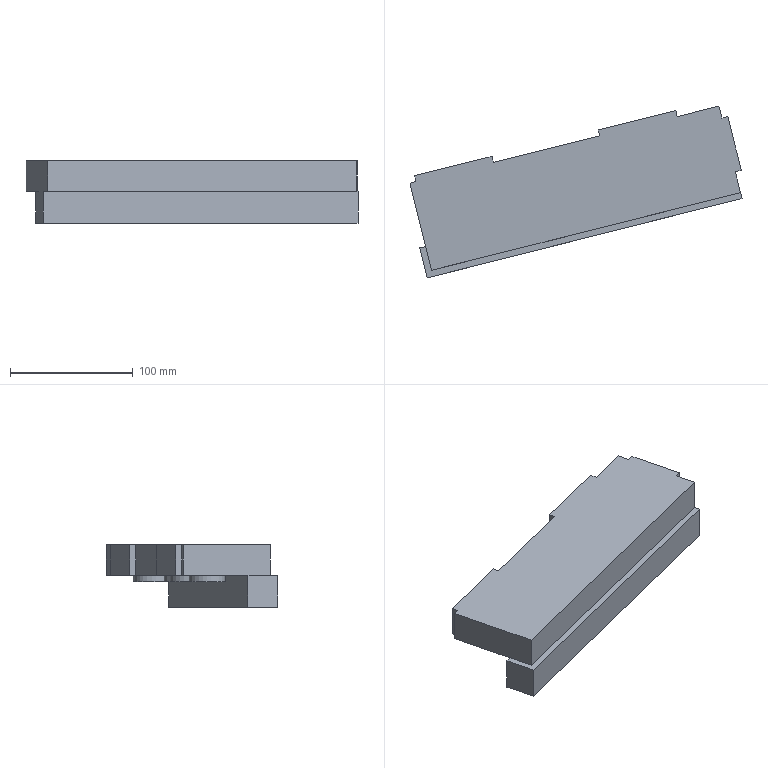Part | NX | features solid 2 | 1 solid | 33 faces | box 270.03 x 139.571 x 51 mm | volume 681907 mm3 | plane 25 | cylinder 5 | spline 3 | commonest cylinder face diameters 30 x5
STEP:
#1=CARTESIAN_POINT('',(-5.928,607.408,20.));
#2=VERTEX_POINT('',#1);
#3=CARTESIAN_POINT('',(9.072,607.408,20.));
#4=DIRECTION('',(0.,0.,-1.));
#5=DIRECTION('',(-1.,0.,0.));
#6=AXIS2_PLACEMENT_3D('',#3,#4,#5);
#7=CIRCLE('',#6,15.);
#8=EDGE_CURVE('',#2,#2,#7,.T.);
#9=ORIENTED_EDGE('',*,*,#8,.F.);
#10=EDGE_LOOP('',(#9));
#11=FACE_BOUND('',#10,.T.);
#12=CARTESIAN_POINT('',(114.072,637.408,20.));
#13=VERTEX_POINT('',#12);
#14=CARTESIAN_POINT('',(129.072,637.408,20.));
#15=DIRECTION('',(0.,0.,-1.));
#16=DIRECTION('',(-1.,0.,0.));
#17=AXIS2_PLACEMENT_3D('',#14,#15,#16);
#18=CIRCLE('',#17,15.);
#19=EDGE_CURVE('',#13,#13,#18,.T.);
#20=ORIENTED_EDGE('',*,*,#19,.F.);
#21=EDGE_LOOP('',(#20));
#22=FACE_BOUND('',#21,.T.);
#23=CARTESIAN_POINT('',(188.432,674.455,20.));
#24=VERTEX_POINT('',#23);
#25=CARTESIAN_POINT('',(154.471,665.988,20.));
#26=VERTEX_POINT('',#25);
#27=CARTESIAN_POINT('',(-67.726,610.588,20.));
#28=DIRECTION('',(0.9703,0.2419,0.));
#29=VECTOR('',#28,1000.);
#30=LINE('',#27,#29);
#31=EDGE_CURVE('',#24,#26,#30,.F.);
#32=ORIENTED_EDGE('',*,*,#31,.F.);
#33=CARTESIAN_POINT('',(190.851,664.752,20.));
#34=VERTEX_POINT('',#33);
#35=CARTESIAN_POINT('',(207.307,598.752,20.));
#36=DIRECTION('',(-0.2419,0.9703,0.));
#37=VECTOR('',#36,1000.);
#38=LINE('',#35,#37);
#39=EDGE_CURVE('',#24,#34,#38,.F.);
#40=ORIENTED_EDGE('',*,*,#39,.T.);
#41=CARTESIAN_POINT('',(195.702,665.962,20.));
#42=VERTEX_POINT('',#41);
#43=CARTESIAN_POINT('',(190.851,664.752,20.));
#44=DIRECTION('',(0.9703,0.2419,0.));
#45=VECTOR('',#44,1000.);
#46=LINE('',#43,#45);
#47=EDGE_CURVE('',#34,#42,#46,.T.);
#48=ORIENTED_EDGE('',*,*,#47,.T.);
#49=CARTESIAN_POINT('',(206.589,622.298,20.));
#50=VERTEX_POINT('',#49);
#51=CARTESIAN_POINT('',(198.122,656.259,20.));
#52=DIRECTION('',(-0.2419,0.9703,0.));
#53=VECTOR('',#52,1000.);
#54=LINE('',#51,#53);
#55=EDGE_CURVE('',#50,#42,#54,.T.);
#56=ORIENTED_EDGE('',*,*,#55,.F.);
#57=CARTESIAN_POINT('',(201.737,621.089,20.));
#58=VERTEX_POINT('',#57);
#59=CARTESIAN_POINT('',(201.737,621.089,20.));
#60=DIRECTION('',(0.9703,0.2419,0.));
#61=VECTOR('',#60,1000.);
#62=LINE('',#59,#61);
#63=EDGE_CURVE('',#58,#50,#62,.T.);
#64=ORIENTED_EDGE('',*,*,#63,.F.);
#65=CARTESIAN_POINT('',(201.108,623.615,20.));
#66=VERTEX_POINT('',#65);
#67=CARTESIAN_POINT('',(193.27,655.049,20.));
#68=DIRECTION('',(-0.2419,0.9703,0.));
#69=VECTOR('',#68,1000.);
#70=LINE('',#67,#69);
#71=EDGE_CURVE('',#58,#66,#70,.T.);
#72=ORIENTED_EDGE('',*,*,#71,.T.);
#73=CARTESIAN_POINT('',(-50.051,560.362,20.));
#74=VERTEX_POINT('',#73);
#75=CARTESIAN_POINT('',(-50.051,560.362,20.));
#76=CARTESIAN_POINT('',(33.671,581.439,20.));
#77=CARTESIAN_POINT('',(117.388,602.531,20.));
#78=CARTESIAN_POINT('',(201.108,623.615,20.));
#79=B_SPLINE_CURVE_WITH_KNOTS('',3,(#75,#76,#77,#78),.UNSPECIFIED.,.F.,.F.,(4,4),(1.461,1.72),.UNSPECIFIED.);
#80=EDGE_CURVE('',#74,#66,#79,.T.);
#81=ORIENTED_EDGE('',*,*,#80,.F.);
#82=CARTESIAN_POINT('',(-62.875,611.797,20.));
#83=VERTEX_POINT('',#82);
#84=CARTESIAN_POINT('',(-45.209,540.945,20.));
#85=DIRECTION('',(0.2419,-0.9703,0.));
#86=VECTOR('',#85,1000.);
#87=LINE('',#84,#86);
#88=EDGE_CURVE('',#74,#83,#87,.F.);
#89=ORIENTED_EDGE('',*,*,#88,.T.);
#90=CARTESIAN_POINT('',(-58.023,613.007,20.));
#91=VERTEX_POINT('',#90);
#92=CARTESIAN_POINT('',(-67.726,610.588,20.));
#93=DIRECTION('',(0.9703,0.2419,0.));
#94=VECTOR('',#93,1000.);
#95=LINE('',#92,#94);
#96=EDGE_CURVE('',#91,#83,#95,.F.);
#97=ORIENTED_EDGE('',*,*,#96,.F.);
#98=CARTESIAN_POINT('',(-59.233,617.858,20.));
#99=VERTEX_POINT('',#98);
#100=CARTESIAN_POINT('',(-58.023,613.007,20.));
#101=DIRECTION('',(-0.2419,0.9703,0.));
#102=VECTOR('',#101,1000.);
#103=LINE('',#100,#102);
#104=EDGE_CURVE('',#91,#99,#103,.T.);
#105=ORIENTED_EDGE('',*,*,#104,.T.);
#106=CARTESIAN_POINT('',(3.836,633.583,20.));
#107=VERTEX_POINT('',#106);
#108=CARTESIAN_POINT('',(-64.084,616.649,20.));
#109=DIRECTION('',(0.9703,0.2419,0.));
#110=VECTOR('',#109,1000.);
#111=LINE('',#108,#110);
#112=EDGE_CURVE('',#99,#107,#111,.T.);
#113=ORIENTED_EDGE('',*,*,#112,.T.);
#114=CARTESIAN_POINT('',(5.046,628.732,20.));
#115=VERTEX_POINT('',#114);
#116=CARTESIAN_POINT('',(5.046,628.732,20.));
#117=DIRECTION('',(-0.2419,0.9703,0.));
#118=VECTOR('',#117,1000.);
#119=LINE('',#116,#118);
#120=EDGE_CURVE('',#115,#107,#119,.T.);
#121=ORIENTED_EDGE('',*,*,#120,.F.);
#122=CARTESIAN_POINT('',(91.402,650.263,20.));
#123=VERTEX_POINT('',#122);
#124=CARTESIAN_POINT('',(-67.726,610.588,20.));
#125=DIRECTION('',(0.9703,0.2419,0.));
#126=VECTOR('',#125,1000.);
#127=LINE('',#124,#126);
#128=EDGE_CURVE('',#123,#115,#127,.F.);
#129=ORIENTED_EDGE('',*,*,#128,.F.);
#130=CARTESIAN_POINT('',(90.193,655.114,20.));
#131=VERTEX_POINT('',#130);
#132=CARTESIAN_POINT('',(91.402,650.263,20.));
#133=DIRECTION('',(-0.2419,0.9703,0.));
#134=VECTOR('',#133,1000.);
#135=LINE('',#132,#134);
#136=EDGE_CURVE('',#123,#131,#135,.T.);
#137=ORIENTED_EDGE('',*,*,#136,.T.);
#138=CARTESIAN_POINT('',(153.262,670.839,20.));
#139=VERTEX_POINT('',#138);
#140=CARTESIAN_POINT('',(129.004,664.791,20.));
#141=DIRECTION('',(0.9703,0.2419,0.));
#142=VECTOR('',#141,1000.);
#143=LINE('',#140,#142);
#144=EDGE_CURVE('',#131,#139,#143,.T.);
#145=ORIENTED_EDGE('',*,*,#144,.T.);
#146=CARTESIAN_POINT('',(154.471,665.988,20.));
#147=DIRECTION('',(-0.2419,0.9703,0.));
#148=VECTOR('',#147,1000.);
#149=LINE('',#146,#148);
#150=EDGE_CURVE('',#26,#139,#149,.T.);
#151=ORIENTED_EDGE('',*,*,#150,.F.);
#152=EDGE_LOOP('',(#32,#40,#48,#56,#64,#72,#81,#89,#97,#105,#113,#121,#129,#137,#145,#151));
#153=FACE_BOUND('',#152,.T.);
#154=CARTESIAN_POINT('',(-35.928,592.408,20.));
#155=VERTEX_POINT('',#154);
#156=CARTESIAN_POINT('',(-20.928,592.408,20.));
#157=DIRECTION('',(0.,0.,-1.));
#158=DIRECTION('',(-1.,0.,0.));
#159=AXIS2_PLACEMENT_3D('',#156,#157,#158);
#160=CIRCLE('',#159,15.);
#161=EDGE_CURVE('',#155,#155,#160,.T.);
#162=ORIENTED_EDGE('',*,*,#161,.F.);
#163=EDGE_LOOP('',(#162));
#164=FACE_BOUND('',#163,.T.);
#165=CARTESIAN_POINT('',(59.072,612.408,20.));
#166=VERTEX_POINT('',#165);
#167=CARTESIAN_POINT('',(74.072,612.408,20.));
#168=DIRECTION('',(0.,0.,-1.));
#169=DIRECTION('',(-1.,0.,0.));
#170=AXIS2_PLACEMENT_3D('',#167,#168,#169);
#171=CIRCLE('',#170,15.);
#172=EDGE_CURVE('',#166,#166,#171,.T.);
#173=ORIENTED_EDGE('',*,*,#172,.F.);
#174=EDGE_LOOP('',(#173));
#175=FACE_BOUND('',#174,.T.);
#176=CARTESIAN_POINT('',(149.072,637.408,20.));
#177=VERTEX_POINT('',#176);
#178=CARTESIAN_POINT('',(164.072,637.408,20.));
#179=DIRECTION('',(0.,0.,-1.));
#180=DIRECTION('',(-1.,0.,0.));
#181=AXIS2_PLACEMENT_3D('',#178,#179,#180);
#182=CIRCLE('',#181,15.);
#183=EDGE_CURVE('',#177,#177,#182,.T.);
#184=ORIENTED_EDGE('',*,*,#183,.F.);
#185=EDGE_LOOP('',(#184));
#186=FACE_BOUND('',#185,.T.);
#187=CARTESIAN_POINT('',(-48.851,534.884,20.));
#188=DIRECTION('',(0.,0.,-1.));
#189=DIRECTION('',(-1.,0.,0.));
#190=AXIS2_PLACEMENT_3D('',#187,#188,#189);
#191=PLANE('',#190);
#192=ADVANCED_FACE('',(#11,#22,#153,#164,#175,#186),#191,.T.);
#193=CARTESIAN_POINT('',(190.851,664.752,45.));
#194=VERTEX_POINT('',#193);
#195=CARTESIAN_POINT('',(188.432,674.455,45.));
#196=VERTEX_POINT('',#195);
#197=CARTESIAN_POINT('',(819.566,-1856.886,45.));
#198=DIRECTION('',(-0.2419,0.9703,0.));
#199=VECTOR('',#198,1000.);
#200=LINE('',#197,#199);
#201=EDGE_CURVE('',#194,#196,#200,.T.);
#202=ORIENTED_EDGE('',*,*,#201,.F.);
#203=CARTESIAN_POINT('',(190.851,664.752,20.));
#204=DIRECTION('',(0.,0.,1.));
#205=VECTOR('',#204,1000.);
#206=LINE('',#203,#205);
#207=EDGE_CURVE('',#34,#194,#206,.T.);
#208=ORIENTED_EDGE('',*,*,#207,.F.);
#209=ORIENTED_EDGE('',*,*,#39,.F.);
#210=CARTESIAN_POINT('',(188.432,674.455,70.));
#211=DIRECTION('',(0.,0.,-1.));
#212=VECTOR('',#211,1000.);
#213=LINE('',#210,#212);
#214=EDGE_CURVE('',#196,#24,#213,.T.);
#215=ORIENTED_EDGE('',*,*,#214,.F.);
#216=EDGE_LOOP('',(#202,#208,#209,#215));
#217=FACE_BOUND('',#216,.T.);
#218=CARTESIAN_POINT('',(819.566,-1856.886,70.));
#219=DIRECTION('',(-0.9703,-0.2419,0.));
#220=DIRECTION('',(0.2419,-0.9703,0.));
#221=AXIS2_PLACEMENT_3D('',#218,#219,#220);
#222=PLANE('',#221);
#223=ADVANCED_FACE('',(#217),#222,.F.);
#224=CARTESIAN_POINT('',(5.046,628.732,45.));
#225=VERTEX_POINT('',#224);
#226=CARTESIAN_POINT('',(91.402,650.263,45.));
#227=VERTEX_POINT('',#226);
#228=CARTESIAN_POINT('',(-334.558,544.059,45.));
#229=DIRECTION('',(0.9703,0.2419,0.));
#230=VECTOR('',#229,1000.);
#231=LINE('',#228,#230);
#232=EDGE_CURVE('',#225,#227,#231,.T.);
#233=ORIENTED_EDGE('',*,*,#232,.T.);
#234=CARTESIAN_POINT('',(91.402,650.263,45.));
#235=DIRECTION('',(0.,0.,1.));
#236=VECTOR('',#235,1000.);
#237=LINE('',#234,#236);
#238=EDGE_CURVE('',#227,#123,#237,.F.);
#239=ORIENTED_EDGE('',*,*,#238,.T.);
#240=ORIENTED_EDGE('',*,*,#128,.T.);
#241=CARTESIAN_POINT('',(5.046,628.732,45.));
#242=DIRECTION('',(0.,0.,-1.));
#243=VECTOR('',#242,1000.);
#244=LINE('',#241,#243);
#245=EDGE_CURVE('',#225,#115,#244,.T.);
#246=ORIENTED_EDGE('',*,*,#245,.F.);
#247=EDGE_LOOP('',(#233,#239,#240,#246));
#248=FACE_BOUND('',#247,.T.);
#249=CARTESIAN_POINT('',(-334.558,544.059,70.));
#250=DIRECTION('',(-0.2419,0.9703,0.));
#251=DIRECTION('',(-0.9703,-0.2419,0.));
#252=AXIS2_PLACEMENT_3D('',#249,#250,#251);
#253=PLANE('',#252);
#254=ADVANCED_FACE('',(#248),#253,.T.);
#255=CARTESIAN_POINT('',(-62.875,611.797,45.));
#256=VERTEX_POINT('',#255);
#257=CARTESIAN_POINT('',(-58.023,613.007,45.));
#258=VERTEX_POINT('',#257);
#259=CARTESIAN_POINT('',(-334.558,544.059,45.));
#260=DIRECTION('',(0.9703,0.2419,0.));
#261=VECTOR('',#260,1000.);
#262=LINE('',#259,#261);
#263=EDGE_CURVE('',#256,#258,#262,.T.);
#264=ORIENTED_EDGE('',*,*,#263,.T.);
#265=CARTESIAN_POINT('',(-58.023,613.007,45.));
#266=DIRECTION('',(0.,0.,1.));
#267=VECTOR('',#266,1000.);
#268=LINE('',#265,#267);
#269=EDGE_CURVE('',#258,#91,#268,.F.);
#270=ORIENTED_EDGE('',*,*,#269,.T.);
#271=ORIENTED_EDGE('',*,*,#96,.T.);
#272=CARTESIAN_POINT('',(-62.875,611.797,70.));
#273=DIRECTION('',(0.,0.,-1.));
#274=VECTOR('',#273,1000.);
#275=LINE('',#272,#274);
#276=EDGE_CURVE('',#256,#83,#275,.T.);
#277=ORIENTED_EDGE('',*,*,#276,.F.);
#278=EDGE_LOOP('',(#264,#270,#271,#277));
#279=FACE_BOUND('',#278,.T.);
#280=CARTESIAN_POINT('',(-334.558,544.059,70.));
#281=DIRECTION('',(-0.2419,0.9703,0.));
#282=DIRECTION('',(-0.9703,-0.2419,0.));
#283=AXIS2_PLACEMENT_3D('',#280,#281,#282);
#284=PLANE('',#283);
#285=ADVANCED_FACE('',(#279),#284,.T.);
#286=CARTESIAN_POINT('',(-54.899,559.142,-6.));
#287=VERTEX_POINT('',#286);
#288=CARTESIAN_POINT('',(-54.899,559.142,20.));
#289=VERTEX_POINT('',#288);
#290=CARTESIAN_POINT('',(-54.899,559.142,9.5));
#291=DIRECTION('',(0.,0.,1.));
#292=VECTOR('',#291,1000.);
#293=LINE('',#290,#292);
#294=EDGE_CURVE('',#287,#289,#293,.T.);
#295=ORIENTED_EDGE('',*,*,#294,.F.);
#296=CARTESIAN_POINT('',(-48.851,534.884,-6.));
#297=VERTEX_POINT('',#296);
#298=CARTESIAN_POINT('',(563.408,-1920.754,-6.));
#299=DIRECTION('',(-0.2419,0.9703,0.));
#300=VECTOR('',#299,1000.);
#301=LINE('',#298,#300);
#302=EDGE_CURVE('',#297,#287,#301,.T.);
#303=ORIENTED_EDGE('',*,*,#302,.F.);
#304=CARTESIAN_POINT('',(-48.851,534.884,20.));
#305=VERTEX_POINT('',#304);
#306=CARTESIAN_POINT('',(-48.851,534.884,70.));
#307=DIRECTION('',(0.,0.,-1.));
#308=VECTOR('',#307,1000.);
#309=LINE('',#306,#308);
#310=EDGE_CURVE('',#305,#297,#309,.T.);
#311=ORIENTED_EDGE('',*,*,#310,.F.);
#312=CARTESIAN_POINT('',(563.408,-1920.754,20.));
#313=DIRECTION('',(-0.2419,0.9703,0.));
#314=VECTOR('',#313,1000.);
#315=LINE('',#312,#314);
#316=EDGE_CURVE('',#289,#305,#315,.F.);
#317=ORIENTED_EDGE('',*,*,#316,.F.);
#318=EDGE_LOOP('',(#295,#303,#311,#317));
#319=FACE_BOUND('',#318,.T.);
#320=CARTESIAN_POINT('',(563.408,-1920.754,70.));
#321=DIRECTION('',(-0.9703,-0.2419,0.));
#322=DIRECTION('',(0.2419,-0.9703,0.));
#323=AXIS2_PLACEMENT_3D('',#320,#321,#322);
#324=PLANE('',#323);
#325=ADVANCED_FACE('',(#319),#324,.T.);
#326=CARTESIAN_POINT('',(154.471,665.988,45.));
#327=VERTEX_POINT('',#326);
#328=CARTESIAN_POINT('',(154.471,665.988,45.));
#329=DIRECTION('',(0.,0.,-1.));
#330=VECTOR('',#329,1000.);
#331=LINE('',#328,#330);
#332=EDGE_CURVE('',#327,#26,#331,.T.);
#333=ORIENTED_EDGE('',*,*,#332,.F.);
#334=CARTESIAN_POINT('',(-334.558,544.059,45.));
#335=DIRECTION('',(0.9703,0.2419,0.));
#336=VECTOR('',#335,1000.);
#337=LINE('',#334,#336);
#338=EDGE_CURVE('',#327,#196,#337,.T.);
#339=ORIENTED_EDGE('',*,*,#338,.T.);
#340=ORIENTED_EDGE('',*,*,#214,.T.);
#341=ORIENTED_EDGE('',*,*,#31,.T.);
#342=EDGE_LOOP('',(#333,#339,#340,#341));
#343=FACE_BOUND('',#342,.T.);
#344=CARTESIAN_POINT('',(-334.558,544.059,70.));
#345=DIRECTION('',(-0.2419,0.9703,0.));
#346=DIRECTION('',(-0.9703,-0.2419,0.));
#347=AXIS2_PLACEMENT_3D('',#344,#345,#346);
#348=PLANE('',#347);
#349=ADVANCED_FACE('',(#343),#348,.T.);
#350=ORIENTED_EDGE('',*,*,#263,.F.);
#351=CARTESIAN_POINT('',(-45.212,540.956,45.));
#352=VERTEX_POINT('',#351);
#353=CARTESIAN_POINT('',(-45.209,540.945,45.));
#354=DIRECTION('',(-0.2419,0.9703,0.));
#355=VECTOR('',#354,1000.);
#356=LINE('',#353,#355);
#357=EDGE_CURVE('',#352,#256,#356,.T.);
#358=ORIENTED_EDGE('',*,*,#357,.F.);
#359=CARTESIAN_POINT('',(205.946,604.209,45.));
#360=VERTEX_POINT('',#359);
#361=CARTESIAN_POINT('',(-45.212,540.956,45.));
#362=CARTESIAN_POINT('',(38.507,562.041,45.));
#363=CARTESIAN_POINT('',(122.227,583.125,45.));
#364=CARTESIAN_POINT('',(205.946,604.209,45.));
#365=B_SPLINE_CURVE_WITH_KNOTS('',3,(#361,#362,#363,#364),.UNSPECIFIED.,.F.,.F.,(4,4),(0.,1.),.UNSPECIFIED.);
#366=EDGE_CURVE('',#352,#360,#365,.T.);
#367=ORIENTED_EDGE('',*,*,#366,.T.);
#368=CARTESIAN_POINT('',(201.737,621.089,45.));
#369=VERTEX_POINT('',#368);
#370=CARTESIAN_POINT('',(819.566,-1856.886,45.));
#371=DIRECTION('',(-0.2419,0.9703,0.));
#372=VECTOR('',#371,1000.);
#373=LINE('',#370,#372);
#374=EDGE_CURVE('',#360,#369,#373,.T.);
#375=ORIENTED_EDGE('',*,*,#374,.T.);
#376=CARTESIAN_POINT('',(206.589,622.298,45.));
#377=VERTEX_POINT('',#376);
#378=CARTESIAN_POINT('',(201.737,621.089,45.));
#379=DIRECTION('',(0.9703,0.2419,0.));
#380=VECTOR('',#379,1000.);
#381=LINE('',#378,#380);
#382=EDGE_CURVE('',#369,#377,#381,.T.);
#383=ORIENTED_EDGE('',*,*,#382,.T.);
#384=CARTESIAN_POINT('',(195.702,665.962,45.));
#385=VERTEX_POINT('',#384);
#386=CARTESIAN_POINT('',(198.122,656.259,45.));
#387=DIRECTION('',(0.2419,-0.9703,0.));
#388=VECTOR('',#387,1000.);
#389=LINE('',#386,#388);
#390=EDGE_CURVE('',#377,#385,#389,.F.);
#391=ORIENTED_EDGE('',*,*,#390,.T.);
#392=CARTESIAN_POINT('',(190.851,664.752,45.));
#393=DIRECTION('',(0.9703,0.2419,0.));
#394=VECTOR('',#393,1000.);
#395=LINE('',#392,#394);
#396=EDGE_CURVE('',#194,#385,#395,.T.);
#397=ORIENTED_EDGE('',*,*,#396,.F.);
#398=ORIENTED_EDGE('',*,*,#201,.T.);
#399=ORIENTED_EDGE('',*,*,#338,.F.);
#400=CARTESIAN_POINT('',(153.262,670.839,45.));
#401=VERTEX_POINT('',#400);
#402=CARTESIAN_POINT('',(154.471,665.988,45.));
#403=DIRECTION('',(-0.2419,0.9703,0.));
#404=VECTOR('',#403,1000.);
#405=LINE('',#402,#404);
#406=EDGE_CURVE('',#327,#401,#405,.T.);
#407=ORIENTED_EDGE('',*,*,#406,.T.);
#408=CARTESIAN_POINT('',(90.193,655.114,45.));
#409=VERTEX_POINT('',#408);
#410=CARTESIAN_POINT('',(129.004,664.791,45.));
#411=DIRECTION('',(0.9703,0.2419,0.));
#412=VECTOR('',#411,1000.);
#413=LINE('',#410,#412);
#414=EDGE_CURVE('',#409,#401,#413,.T.);
#415=ORIENTED_EDGE('',*,*,#414,.F.);
#416=CARTESIAN_POINT('',(91.402,650.263,45.));
#417=DIRECTION('',(-0.2419,0.9703,0.));
#418=VECTOR('',#417,1000.);
#419=LINE('',#416,#418);
#420=EDGE_CURVE('',#227,#409,#419,.T.);
#421=ORIENTED_EDGE('',*,*,#420,.F.);
#422=ORIENTED_EDGE('',*,*,#232,.F.);
#423=CARTESIAN_POINT('',(3.836,633.583,45.));
#424=VERTEX_POINT('',#423);
#425=CARTESIAN_POINT('',(5.046,628.732,45.));
#426=DIRECTION('',(-0.2419,0.9703,0.));
#427=VECTOR('',#426,1000.);
#428=LINE('',#425,#427);
#429=EDGE_CURVE('',#225,#424,#428,.T.);
#430=ORIENTED_EDGE('',*,*,#429,.T.);
#431=CARTESIAN_POINT('',(-59.233,617.858,45.));
#432=VERTEX_POINT('',#431);
#433=CARTESIAN_POINT('',(-64.084,616.649,45.));
#434=DIRECTION('',(0.9703,0.2419,0.));
#435=VECTOR('',#434,1000.);
#436=LINE('',#433,#435);
#437=EDGE_CURVE('',#432,#424,#436,.T.);
#438=ORIENTED_EDGE('',*,*,#437,.F.);
#439=CARTESIAN_POINT('',(-58.023,613.007,45.));
#440=DIRECTION('',(-0.2419,0.9703,0.));
#441=VECTOR('',#440,1000.);
#442=LINE('',#439,#441);
#443=EDGE_CURVE('',#258,#432,#442,.T.);
#444=ORIENTED_EDGE('',*,*,#443,.F.);
#445=EDGE_LOOP('',(#350,#358,#367,#375,#383,#391,#397,#398,#399,#407,#415,#421,#422,#430,#438,#444));
#446=FACE_BOUND('',#445,.T.);
#447=CARTESIAN_POINT('',(68.11,-778.743,45.));
#448=DIRECTION('',(0.,0.,1.));
#449=DIRECTION('',(1.,0.,0.));
#450=AXIS2_PLACEMENT_3D('',#447,#448,#449);
#451=PLANE('',#450);
#452=ADVANCED_FACE('',(#446),#451,.T.);
#453=CARTESIAN_POINT('',(-45.212,540.956,20.));
#454=VERTEX_POINT('',#453);
#455=CARTESIAN_POINT('',(-45.212,540.956,42.5));
#456=DIRECTION('',(0.,0.,-1.));
#457=VECTOR('',#456,1000.);
#458=LINE('',#455,#457);
#459=EDGE_CURVE('',#454,#352,#458,.F.);
#460=ORIENTED_EDGE('',*,*,#459,.F.);
#461=CARTESIAN_POINT('',(205.946,604.209,20.));
#462=VERTEX_POINT('',#461);
#463=CARTESIAN_POINT('',(205.946,604.209,20.));
#464=CARTESIAN_POINT('',(122.227,583.125,20.));
#465=CARTESIAN_POINT('',(38.509,562.033,20.));
#466=CARTESIAN_POINT('',(-45.212,540.956,20.));
#467=B_SPLINE_CURVE_WITH_KNOTS('',3,(#463,#464,#465,#466),.UNSPECIFIED.,.F.,.F.,(4,4),(1.061,1.32),.UNSPECIFIED.);
#468=EDGE_CURVE('',#454,#462,#467,.F.);
#469=ORIENTED_EDGE('',*,*,#468,.T.);
#470=CARTESIAN_POINT('',(205.946,604.209,15.));
#471=DIRECTION('',(0.,0.,-1.));
#472=VECTOR('',#471,1000.);
#473=LINE('',#470,#472);
#474=EDGE_CURVE('',#462,#360,#473,.F.);
#475=ORIENTED_EDGE('',*,*,#474,.T.);
#476=ORIENTED_EDGE('',*,*,#366,.F.);
#477=EDGE_LOOP('',(#460,#469,#475,#476));
#478=FACE_BOUND('',#477,.T.);
#479=CARTESIAN_POINT('',(-45.212,540.956,45.));
#480=CARTESIAN_POINT('',(-45.212,540.956,20.));
#481=CARTESIAN_POINT('',(38.51,562.034,45.));
#482=CARTESIAN_POINT('',(38.51,562.034,20.));
#483=CARTESIAN_POINT('',(122.226,583.125,45.));
#484=CARTESIAN_POINT('',(122.226,583.125,20.));
#485=CARTESIAN_POINT('',(205.946,604.209,45.));
#486=CARTESIAN_POINT('',(205.946,604.209,20.));
#487=B_SPLINE_SURFACE_WITH_KNOTS('',3,1,((#479,#480),(#481,#482),(#483,#484),(#485,#486)),.SURF_OF_LINEAR_EXTRUSION.,.F.,.F.,.F.,(4,4),(2,2),(0.01891,0.9963),(0.,1.),.PIECEWISE_BEZIER_KNOTS.);
#488=ADVANCED_FACE('',(#478),#487,.F.);
#489=CARTESIAN_POINT('',(201.108,623.615,-6.));
#490=VERTEX_POINT('',#489);
#491=CARTESIAN_POINT('',(201.108,623.615,19.5));
#492=DIRECTION('',(0.,0.,1.));
#493=VECTOR('',#492,1000.);
#494=LINE('',#491,#493);
#495=EDGE_CURVE('',#490,#66,#494,.T.);
#496=ORIENTED_EDGE('',*,*,#495,.T.);
#497=ORIENTED_EDGE('',*,*,#71,.F.);
#498=CARTESIAN_POINT('',(201.737,621.089,20.));
#499=DIRECTION('',(0.,0.,-1.));
#500=VECTOR('',#499,1000.);
#501=LINE('',#498,#500);
#502=EDGE_CURVE('',#58,#369,#501,.F.);
#503=ORIENTED_EDGE('',*,*,#502,.T.);
#504=ORIENTED_EDGE('',*,*,#374,.F.);
#505=ORIENTED_EDGE('',*,*,#474,.F.);
#506=CARTESIAN_POINT('',(207.156,599.358,20.));
#507=VERTEX_POINT('',#506);
#508=CARTESIAN_POINT('',(207.307,598.752,20.));
#509=DIRECTION('',(0.2419,-0.9703,0.));
#510=VECTOR('',#509,1000.);
#511=LINE('',#508,#510);
#512=EDGE_CURVE('',#507,#462,#511,.F.);
#513=ORIENTED_EDGE('',*,*,#512,.F.);
#514=CARTESIAN_POINT('',(207.156,599.358,-6.));
#515=VERTEX_POINT('',#514);
#516=CARTESIAN_POINT('',(207.156,599.358,2.5));
#517=DIRECTION('',(0.,0.,-1.));
#518=VECTOR('',#517,1000.);
#519=LINE('',#516,#518);
#520=EDGE_CURVE('',#507,#515,#519,.T.);
#521=ORIENTED_EDGE('',*,*,#520,.T.);
#522=CARTESIAN_POINT('',(819.566,-1856.886,-6.));
#523=DIRECTION('',(-0.2419,0.9703,0.));
#524=VECTOR('',#523,1000.);
#525=LINE('',#522,#524);
#526=EDGE_CURVE('',#515,#490,#525,.T.);
#527=ORIENTED_EDGE('',*,*,#526,.T.);
#528=EDGE_LOOP('',(#496,#497,#503,#504,#505,#513,#521,#527));
#529=FACE_BOUND('',#528,.T.);
#530=CARTESIAN_POINT('',(819.566,-1856.886,70.));
#531=DIRECTION('',(-0.9703,-0.2419,0.));
#532=DIRECTION('',(0.2419,-0.9703,0.));
#533=AXIS2_PLACEMENT_3D('',#530,#531,#532);
#534=PLANE('',#533);
#535=ADVANCED_FACE('',(#529),#534,.F.);
#536=ORIENTED_EDGE('',*,*,#302,.T.);
#537=CARTESIAN_POINT('',(-54.899,559.142,-6.));
#538=CARTESIAN_POINT('',(30.438,580.627,-6.));
#539=CARTESIAN_POINT('',(115.772,602.124,-6.));
#540=CARTESIAN_POINT('',(201.108,623.615,-6.));
#541=B_SPLINE_CURVE_WITH_KNOTS('',3,(#537,#538,#539,#540),.UNSPECIFIED.,.F.,.F.,(4,4),(0.,0.264),.UNSPECIFIED.);
#542=EDGE_CURVE('',#287,#490,#541,.T.);
#543=ORIENTED_EDGE('',*,*,#542,.T.);
#544=ORIENTED_EDGE('',*,*,#526,.F.);
#545=CARTESIAN_POINT('',(207.156,599.358,-6.));
#546=CARTESIAN_POINT('',(121.82,577.867,-6.));
#547=CARTESIAN_POINT('',(36.486,556.369,-6.));
#548=CARTESIAN_POINT('',(-48.851,534.884,-6.));
#549=B_SPLINE_CURVE_WITH_KNOTS('',3,(#545,#546,#547,#548),.UNSPECIFIED.,.F.,.F.,(4,4),(1.823,2.087),.UNSPECIFIED.);
#550=EDGE_CURVE('',#297,#515,#549,.F.);
#551=ORIENTED_EDGE('',*,*,#550,.F.);
#552=EDGE_LOOP('',(#536,#543,#544,#551));
#553=FACE_BOUND('',#552,.T.);
#554=CARTESIAN_POINT('',(68.11,-778.743,-6.));
#555=DIRECTION('',(0.,0.,1.));
#556=DIRECTION('',(1.,0.,0.));
#557=AXIS2_PLACEMENT_3D('',#554,#555,#556);
#558=PLANE('',#557);
#559=ADVANCED_FACE('',(#553),#558,.F.);
#560=CARTESIAN_POINT('',(207.156,599.358,20.));
#561=CARTESIAN_POINT('',(121.82,577.867,20.));
#562=CARTESIAN_POINT('',(36.486,556.369,20.));
#563=CARTESIAN_POINT('',(-48.851,534.884,20.));
#564=B_SPLINE_CURVE_WITH_KNOTS('',3,(#560,#561,#562,#563),.UNSPECIFIED.,.F.,.F.,(4,4),(1.875,2.139),.UNSPECIFIED.);
#565=EDGE_CURVE('',#305,#507,#564,.F.);
#566=ORIENTED_EDGE('',*,*,#565,.F.);
#567=ORIENTED_EDGE('',*,*,#310,.T.);
#568=ORIENTED_EDGE('',*,*,#550,.T.);
#569=ORIENTED_EDGE('',*,*,#520,.F.);
#570=EDGE_LOOP('',(#566,#567,#568,#569));
#571=FACE_BOUND('',#570,.T.);
#572=CARTESIAN_POINT('',(-48.851,534.884,20.));
#573=CARTESIAN_POINT('',(-48.851,534.884,-6.));
#574=CARTESIAN_POINT('',(36.486,556.369,20.));
#575=CARTESIAN_POINT('',(36.486,556.369,-6.));
#576=CARTESIAN_POINT('',(121.82,577.867,20.));
#577=CARTESIAN_POINT('',(121.82,577.867,-6.));
#578=CARTESIAN_POINT('',(207.156,599.358,20.));
#579=CARTESIAN_POINT('',(207.156,599.358,-6.));
#580=B_SPLINE_SURFACE_WITH_KNOTS('',3,1,((#572,#573),(#574,#575),(#576,#577),(#578,#579)),.SURF_OF_LINEAR_EXTRUSION.,.F.,.F.,.F.,(4,4),(2,2),(0.7724,0.9978),(0.,1.),.PIECEWISE_BEZIER_KNOTS.);
#581=ADVANCED_FACE('',(#571),#580,.F.);
#582=CARTESIAN_POINT('',(-44.,536.094,20.));
#583=DIRECTION('',(0.2419,-0.9703,0.));
#584=VECTOR('',#583,1000.);
#585=LINE('',#582,#584);
#586=EDGE_CURVE('',#454,#74,#585,.F.);
#587=ORIENTED_EDGE('',*,*,#586,.T.);
#588=CARTESIAN_POINT('',(-50.051,560.362,20.));
#589=CARTESIAN_POINT('',(-51.667,559.955,20.));
#590=CARTESIAN_POINT('',(-53.283,559.549,20.));
#591=CARTESIAN_POINT('',(-54.899,559.142,20.));
#592=B_SPLINE_CURVE_WITH_KNOTS('',3,(#588,#589,#590,#591),.UNSPECIFIED.,.F.,.F.,(4,4),(0.,0.005),.UNSPECIFIED.);
#593=EDGE_CURVE('',#74,#289,#592,.T.);
#594=ORIENTED_EDGE('',*,*,#593,.T.);
#595=ORIENTED_EDGE('',*,*,#316,.T.);
#596=ORIENTED_EDGE('',*,*,#565,.T.);
#597=ORIENTED_EDGE('',*,*,#512,.T.);
#598=ORIENTED_EDGE('',*,*,#468,.F.);
#599=EDGE_LOOP('',(#587,#594,#595,#596,#597,#598));
#600=FACE_BOUND('',#599,.T.);
#601=CARTESIAN_POINT('',(-48.851,534.884,20.));
#602=DIRECTION('',(0.,0.,1.));
#603=DIRECTION('',(1.,0.,0.));
#604=AXIS2_PLACEMENT_3D('',#601,#602,#603);
#605=PLANE('',#604);
#606=ADVANCED_FACE('',(#600),#605,.T.);
#607=ORIENTED_EDGE('',*,*,#88,.F.);
#608=ORIENTED_EDGE('',*,*,#586,.F.);
#609=ORIENTED_EDGE('',*,*,#459,.T.);
#610=ORIENTED_EDGE('',*,*,#357,.T.);
#611=ORIENTED_EDGE('',*,*,#276,.T.);
#612=EDGE_LOOP('',(#607,#608,#609,#610,#611));
#613=FACE_BOUND('',#612,.T.);
#614=CARTESIAN_POINT('',(-45.209,540.945,70.));
#615=DIRECTION('',(-0.9703,-0.2419,0.));
#616=DIRECTION('',(0.2419,-0.9703,0.));
#617=AXIS2_PLACEMENT_3D('',#614,#615,#616);
#618=PLANE('',#617);
#619=ADVANCED_FACE('',(#613),#618,.T.);
#620=ORIENTED_EDGE('',*,*,#495,.F.);
#621=ORIENTED_EDGE('',*,*,#542,.F.);
#622=ORIENTED_EDGE('',*,*,#294,.T.);
#623=ORIENTED_EDGE('',*,*,#593,.F.);
#624=ORIENTED_EDGE('',*,*,#80,.T.);
#625=EDGE_LOOP('',(#620,#621,#622,#623,#624));
#626=FACE_BOUND('',#625,.T.);
#627=CARTESIAN_POINT('',(-54.899,559.142,-6.));
#628=CARTESIAN_POINT('',(-54.899,559.142,20.));
#629=CARTESIAN_POINT('',(30.444,580.628,-6.));
#630=CARTESIAN_POINT('',(30.444,580.628,20.));
#631=CARTESIAN_POINT('',(115.771,602.124,-6.));
#632=CARTESIAN_POINT('',(115.771,602.124,20.));
#633=CARTESIAN_POINT('',(201.108,623.615,-6.));
#634=CARTESIAN_POINT('',(201.108,623.615,20.));
#635=B_SPLINE_SURFACE_WITH_KNOTS('',3,1,((#627,#628),(#629,#630),(#631,#632),(#633,#634)),.SURF_OF_LINEAR_EXTRUSION.,.F.,.F.,.F.,(4,4),(2,2),(0.000217,1.),(0.,1.),.PIECEWISE_BEZIER_KNOTS.);
#636=ADVANCED_FACE('',(#626),#635,.F.);
#637=CARTESIAN_POINT('',(3.836,633.583,45.));
#638=DIRECTION('',(0.,0.,-1.));
#639=VECTOR('',#638,1000.);
#640=LINE('',#637,#639);
#641=EDGE_CURVE('',#424,#107,#640,.T.);
#642=ORIENTED_EDGE('',*,*,#641,.F.);
#643=ORIENTED_EDGE('',*,*,#429,.F.);
#644=ORIENTED_EDGE('',*,*,#245,.T.);
#645=ORIENTED_EDGE('',*,*,#120,.T.);
#646=EDGE_LOOP('',(#642,#643,#644,#645));
#647=FACE_BOUND('',#646,.T.);
#648=CARTESIAN_POINT('',(5.046,628.732,45.));
#649=DIRECTION('',(0.9703,0.2419,0.));
#650=DIRECTION('',(-0.2419,0.9703,0.));
#651=AXIS2_PLACEMENT_3D('',#648,#649,#650);
#652=PLANE('',#651);
#653=ADVANCED_FACE('',(#647),#652,.T.);
#654=CARTESIAN_POINT('',(-59.233,617.858,45.));
#655=DIRECTION('',(0.,0.,1.));
#656=VECTOR('',#655,1000.);
#657=LINE('',#654,#656);
#658=EDGE_CURVE('',#432,#99,#657,.F.);
#659=ORIENTED_EDGE('',*,*,#658,.T.);
#660=ORIENTED_EDGE('',*,*,#104,.F.);
#661=ORIENTED_EDGE('',*,*,#269,.F.);
#662=ORIENTED_EDGE('',*,*,#443,.T.);
#663=EDGE_LOOP('',(#659,#660,#661,#662));
#664=FACE_BOUND('',#663,.T.);
#665=CARTESIAN_POINT('',(-58.023,613.007,45.));
#666=DIRECTION('',(0.9703,0.2419,0.));
#667=DIRECTION('',(-0.2419,0.9703,0.));
#668=AXIS2_PLACEMENT_3D('',#665,#666,#667);
#669=PLANE('',#668);
#670=ADVANCED_FACE('',(#664),#669,.F.);
#671=ORIENTED_EDGE('',*,*,#641,.T.);
#672=ORIENTED_EDGE('',*,*,#112,.F.);
#673=ORIENTED_EDGE('',*,*,#658,.F.);
#674=ORIENTED_EDGE('',*,*,#437,.T.);
#675=EDGE_LOOP('',(#671,#672,#673,#674));
#676=FACE_BOUND('',#675,.T.);
#677=CARTESIAN_POINT('',(-64.084,616.649,45.));
#678=DIRECTION('',(0.2419,-0.9703,0.));
#679=DIRECTION('',(0.,0.,-1.));
#680=AXIS2_PLACEMENT_3D('',#677,#678,#679);
#681=PLANE('',#680);
#682=ADVANCED_FACE('',(#676),#681,.F.);
#683=CARTESIAN_POINT('',(153.262,670.839,45.));
#684=DIRECTION('',(0.,0.,-1.));
#685=VECTOR('',#684,1000.);
#686=LINE('',#683,#685);
#687=EDGE_CURVE('',#401,#139,#686,.T.);
#688=ORIENTED_EDGE('',*,*,#687,.F.);
#689=ORIENTED_EDGE('',*,*,#406,.F.);
#690=ORIENTED_EDGE('',*,*,#332,.T.);
#691=ORIENTED_EDGE('',*,*,#150,.T.);
#692=EDGE_LOOP('',(#688,#689,#690,#691));
#693=FACE_BOUND('',#692,.T.);
#694=CARTESIAN_POINT('',(154.471,665.988,45.));
#695=DIRECTION('',(0.9703,0.2419,0.));
#696=DIRECTION('',(-0.2419,0.9703,0.));
#697=AXIS2_PLACEMENT_3D('',#694,#695,#696);
#698=PLANE('',#697);
#699=ADVANCED_FACE('',(#693),#698,.T.);
#700=CARTESIAN_POINT('',(90.193,655.114,45.));
#701=DIRECTION('',(0.,0.,1.));
#702=VECTOR('',#701,1000.);
#703=LINE('',#700,#702);
#704=EDGE_CURVE('',#409,#131,#703,.F.);
#705=ORIENTED_EDGE('',*,*,#704,.T.);
#706=ORIENTED_EDGE('',*,*,#136,.F.);
#707=ORIENTED_EDGE('',*,*,#238,.F.);
#708=ORIENTED_EDGE('',*,*,#420,.T.);
#709=EDGE_LOOP('',(#705,#706,#707,#708));
#710=FACE_BOUND('',#709,.T.);
#711=CARTESIAN_POINT('',(91.402,650.263,45.));
#712=DIRECTION('',(0.9703,0.2419,0.));
#713=DIRECTION('',(-0.2419,0.9703,0.));
#714=AXIS2_PLACEMENT_3D('',#711,#712,#713);
#715=PLANE('',#714);
#716=ADVANCED_FACE('',(#710),#715,.F.);
#717=ORIENTED_EDGE('',*,*,#687,.T.);
#718=ORIENTED_EDGE('',*,*,#144,.F.);
#719=ORIENTED_EDGE('',*,*,#704,.F.);
#720=ORIENTED_EDGE('',*,*,#414,.T.);
#721=EDGE_LOOP('',(#717,#718,#719,#720));
#722=FACE_BOUND('',#721,.T.);
#723=CARTESIAN_POINT('',(129.004,664.791,45.));
#724=DIRECTION('',(0.2419,-0.9703,0.));
#725=DIRECTION('',(0.,0.,-1.));
#726=AXIS2_PLACEMENT_3D('',#723,#724,#725);
#727=PLANE('',#726);
#728=ADVANCED_FACE('',(#722),#727,.F.);
#729=CARTESIAN_POINT('',(195.702,665.962,20.));
#730=DIRECTION('',(0.,0.,1.));
#731=VECTOR('',#730,1000.);
#732=LINE('',#729,#731);
#733=EDGE_CURVE('',#42,#385,#732,.T.);
#734=ORIENTED_EDGE('',*,*,#733,.F.);
#735=ORIENTED_EDGE('',*,*,#47,.F.);
#736=ORIENTED_EDGE('',*,*,#207,.T.);
#737=ORIENTED_EDGE('',*,*,#396,.T.);
#738=EDGE_LOOP('',(#734,#735,#736,#737));
#739=FACE_BOUND('',#738,.T.);
#740=CARTESIAN_POINT('',(190.851,664.752,20.));
#741=DIRECTION('',(-0.2419,0.9703,0.));
#742=DIRECTION('',(-0.9703,-0.2419,0.));
#743=AXIS2_PLACEMENT_3D('',#740,#741,#742);
#744=PLANE('',#743);
#745=ADVANCED_FACE('',(#739),#744,.T.);
#746=CARTESIAN_POINT('',(206.589,622.298,20.));
#747=DIRECTION('',(0.,0.,-1.));
#748=VECTOR('',#747,1000.);
#749=LINE('',#746,#748);
#750=EDGE_CURVE('',#50,#377,#749,.F.);
#751=ORIENTED_EDGE('',*,*,#750,.T.);
#752=ORIENTED_EDGE('',*,*,#382,.F.);
#753=ORIENTED_EDGE('',*,*,#502,.F.);
#754=ORIENTED_EDGE('',*,*,#63,.T.);
#755=EDGE_LOOP('',(#751,#752,#753,#754));
#756=FACE_BOUND('',#755,.T.);
#757=CARTESIAN_POINT('',(201.737,621.089,20.));
#758=DIRECTION('',(-0.2419,0.9703,0.));
#759=DIRECTION('',(-0.9703,-0.2419,0.));
#760=AXIS2_PLACEMENT_3D('',#757,#758,#759);
#761=PLANE('',#760);
#762=ADVANCED_FACE('',(#756),#761,.F.);
#763=ORIENTED_EDGE('',*,*,#733,.T.);
#764=ORIENTED_EDGE('',*,*,#390,.F.);
#765=ORIENTED_EDGE('',*,*,#750,.F.);
#766=ORIENTED_EDGE('',*,*,#55,.T.);
#767=EDGE_LOOP('',(#763,#764,#765,#766));
#768=FACE_BOUND('',#767,.T.);
#769=CARTESIAN_POINT('',(198.122,656.259,20.));
#770=DIRECTION('',(-0.9703,-0.2419,0.));
#771=DIRECTION('',(0.,0.,1.));
#772=AXIS2_PLACEMENT_3D('',#769,#770,#771);
#773=PLANE('',#772);
#774=ADVANCED_FACE('',(#768),#773,.F.);
#775=CARTESIAN_POINT('',(-5.928,592.408,15.));
#776=VERTEX_POINT('',#775);
#777=CARTESIAN_POINT('',(-20.928,592.408,15.));
#778=DIRECTION('',(0.,0.,-1.));
#779=DIRECTION('',(1.,0.,0.));
#780=AXIS2_PLACEMENT_3D('',#777,#778,#779);
#781=CIRCLE('',#780,15.);
#782=EDGE_CURVE('',#776,#776,#781,.T.);
#783=ORIENTED_EDGE('',*,*,#782,.F.);
#784=EDGE_LOOP('',(#783));
#785=FACE_BOUND('',#784,.T.);
#786=ORIENTED_EDGE('',*,*,#161,.T.);
#787=EDGE_LOOP('',(#786));
#788=FACE_BOUND('',#787,.T.);
#789=CARTESIAN_POINT('',(-20.928,592.408,15.));
#790=DIRECTION('',(0.,0.,1.));
#791=DIRECTION('',(1.,0.,0.));
#792=AXIS2_PLACEMENT_3D('',#789,#790,#791);
#793=CYLINDRICAL_SURFACE('',#792,15.);
#794=ADVANCED_FACE('',(#785,#788),#793,.T.);
#795=ORIENTED_EDGE('',*,*,#782,.T.);
#796=EDGE_LOOP('',(#795));
#797=FACE_BOUND('',#796,.T.);
#798=CARTESIAN_POINT('',(-20.928,592.408,15.));
#799=DIRECTION('',(0.,0.,-1.));
#800=DIRECTION('',(-1.,0.,0.));
#801=AXIS2_PLACEMENT_3D('',#798,#799,#800);
#802=PLANE('',#801);
#803=ADVANCED_FACE('',(#797),#802,.T.);
#804=CARTESIAN_POINT('',(144.072,637.408,15.));
#805=VERTEX_POINT('',#804);
#806=CARTESIAN_POINT('',(129.072,637.408,15.));
#807=DIRECTION('',(0.,0.,-1.));
#808=DIRECTION('',(1.,0.,0.));
#809=AXIS2_PLACEMENT_3D('',#806,#807,#808);
#810=CIRCLE('',#809,15.);
#811=EDGE_CURVE('',#805,#805,#810,.T.);
#812=ORIENTED_EDGE('',*,*,#811,.F.);
#813=EDGE_LOOP('',(#812));
#814=FACE_BOUND('',#813,.T.);
#815=ORIENTED_EDGE('',*,*,#19,.T.);
#816=EDGE_LOOP('',(#815));
#817=FACE_BOUND('',#816,.T.);
#818=CARTESIAN_POINT('',(129.072,637.408,15.));
#819=DIRECTION('',(0.,0.,1.));
#820=DIRECTION('',(1.,0.,0.));
#821=AXIS2_PLACEMENT_3D('',#818,#819,#820);
#822=CYLINDRICAL_SURFACE('',#821,15.);
#823=ADVANCED_FACE('',(#814,#817),#822,.T.);
#824=ORIENTED_EDGE('',*,*,#811,.T.);
#825=EDGE_LOOP('',(#824));
#826=FACE_BOUND('',#825,.T.);
#827=CARTESIAN_POINT('',(129.072,637.408,15.));
#828=DIRECTION('',(0.,0.,-1.));
#829=DIRECTION('',(-1.,0.,0.));
#830=AXIS2_PLACEMENT_3D('',#827,#828,#829);
#831=PLANE('',#830);
#832=ADVANCED_FACE('',(#826),#831,.T.);
#833=CARTESIAN_POINT('',(89.072,612.408,15.));
#834=VERTEX_POINT('',#833);
#835=CARTESIAN_POINT('',(74.072,612.408,15.));
#836=DIRECTION('',(0.,0.,-1.));
#837=DIRECTION('',(1.,0.,0.));
#838=AXIS2_PLACEMENT_3D('',#835,#836,#837);
#839=CIRCLE('',#838,15.);
#840=EDGE_CURVE('',#834,#834,#839,.T.);
#841=ORIENTED_EDGE('',*,*,#840,.F.);
#842=EDGE_LOOP('',(#841));
#843=FACE_BOUND('',#842,.T.);
#844=ORIENTED_EDGE('',*,*,#172,.T.);
#845=EDGE_LOOP('',(#844));
#846=FACE_BOUND('',#845,.T.);
#847=CARTESIAN_POINT('',(74.072,612.408,15.));
#848=DIRECTION('',(0.,0.,1.));
#849=DIRECTION('',(1.,0.,0.));
#850=AXIS2_PLACEMENT_3D('',#847,#848,#849);
#851=CYLINDRICAL_SURFACE('',#850,15.);
#852=ADVANCED_FACE('',(#843,#846),#851,.T.);
#853=ORIENTED_EDGE('',*,*,#840,.T.);
#854=EDGE_LOOP('',(#853));
#855=FACE_BOUND('',#854,.T.);
#856=CARTESIAN_POINT('',(74.072,612.408,15.));
#857=DIRECTION('',(0.,0.,-1.));
#858=DIRECTION('',(-1.,0.,0.));
#859=AXIS2_PLACEMENT_3D('',#856,#857,#858);
#860=PLANE('',#859);
#861=ADVANCED_FACE('',(#855),#860,.T.);
#862=CARTESIAN_POINT('',(24.072,607.408,15.));
#863=VERTEX_POINT('',#862);
#864=CARTESIAN_POINT('',(9.072,607.408,15.));
#865=DIRECTION('',(0.,0.,-1.));
#866=DIRECTION('',(1.,0.,0.));
#867=AXIS2_PLACEMENT_3D('',#864,#865,#866);
#868=CIRCLE('',#867,15.);
#869=EDGE_CURVE('',#863,#863,#868,.T.);
#870=ORIENTED_EDGE('',*,*,#869,.F.);
#871=EDGE_LOOP('',(#870));
#872=FACE_BOUND('',#871,.T.);
#873=ORIENTED_EDGE('',*,*,#8,.T.);
#874=EDGE_LOOP('',(#873));
#875=FACE_BOUND('',#874,.T.);
#876=CARTESIAN_POINT('',(9.072,607.408,15.));
#877=DIRECTION('',(0.,0.,1.));
#878=DIRECTION('',(1.,0.,0.));
#879=AXIS2_PLACEMENT_3D('',#876,#877,#878);
#880=CYLINDRICAL_SURFACE('',#879,15.);
#881=ADVANCED_FACE('',(#872,#875),#880,.T.);
#882=ORIENTED_EDGE('',*,*,#869,.T.);
#883=EDGE_LOOP('',(#882));
#884=FACE_BOUND('',#883,.T.);
#885=CARTESIAN_POINT('',(9.072,607.408,15.));
#886=DIRECTION('',(0.,0.,-1.));
#887=DIRECTION('',(-1.,0.,0.));
#888=AXIS2_PLACEMENT_3D('',#885,#886,#887);
#889=PLANE('',#888);
#890=ADVANCED_FACE('',(#884),#889,.T.);
#891=CARTESIAN_POINT('',(179.072,637.408,15.));
#892=VERTEX_POINT('',#891);
#893=CARTESIAN_POINT('',(164.072,637.408,15.));
#894=DIRECTION('',(0.,0.,-1.));
#895=DIRECTION('',(1.,0.,0.));
#896=AXIS2_PLACEMENT_3D('',#893,#894,#895);
#897=CIRCLE('',#896,15.);
#898=EDGE_CURVE('',#892,#892,#897,.T.);
#899=ORIENTED_EDGE('',*,*,#898,.F.);
#900=EDGE_LOOP('',(#899));
#901=FACE_BOUND('',#900,.T.);
#902=ORIENTED_EDGE('',*,*,#183,.T.);
#903=EDGE_LOOP('',(#902));
#904=FACE_BOUND('',#903,.T.);
#905=CARTESIAN_POINT('',(164.072,637.408,15.));
#906=DIRECTION('',(0.,0.,1.));
#907=DIRECTION('',(1.,0.,0.));
#908=AXIS2_PLACEMENT_3D('',#905,#906,#907);
#909=CYLINDRICAL_SURFACE('',#908,15.);
#910=ADVANCED_FACE('',(#901,#904),#909,.T.);
#911=ORIENTED_EDGE('',*,*,#898,.T.);
#912=EDGE_LOOP('',(#911));
#913=FACE_BOUND('',#912,.T.);
#914=CARTESIAN_POINT('',(164.072,637.408,15.));
#915=DIRECTION('',(0.,0.,-1.));
#916=DIRECTION('',(-1.,0.,0.));
#917=AXIS2_PLACEMENT_3D('',#914,#915,#916);
#918=PLANE('',#917);
#919=ADVANCED_FACE('',(#913),#918,.T.);
#920=CLOSED_SHELL('',(#192,#223,#254,#285,#325,#349,#452,#488,#535,#559,#581,#606,#619,#636,#653,#670,#682,#699,#716,#728,#745,#762,#774,#794,#803,#823,#832,#852,#861,#881,#890,#910,#919));
#921=MANIFOLD_SOLID_BREP('',#920);
#922=(LENGTH_UNIT()NAMED_UNIT(*)SI_UNIT(.MILLI.,.METRE.));
#923=UNCERTAINTY_MEASURE_WITH_UNIT(LENGTH_MEASURE(0.0508),#922,'','');
#924=(NAMED_UNIT(*)PLANE_ANGLE_UNIT()SI_UNIT($,.RADIAN.));
#925=(NAMED_UNIT(*)SI_UNIT($,.STERADIAN.)SOLID_ANGLE_UNIT());
#926=(GEOMETRIC_REPRESENTATION_CONTEXT(3)GLOBAL_UNCERTAINTY_ASSIGNED_CONTEXT((#923))GLOBAL_UNIT_ASSIGNED_CONTEXT((#922,#924,#925))REPRESENTATION_CONTEXT('',''));
#927=ADVANCED_BREP_SHAPE_REPRESENTATION('',(#921),#926);